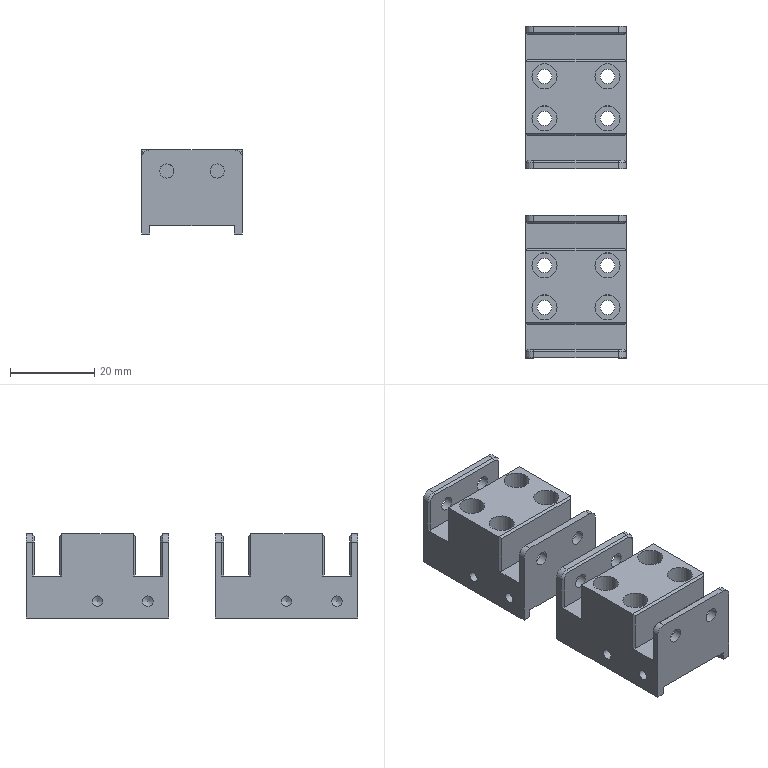CAM job | NX | 3-axis milling, drilling | part box 24 x 79 x 20 mm | stock box 25 x 84 x 25 mm
Tools:
number,name,description,diameter,corner_radius,flute_length,length,flutes
4,D4,平底铣刀-粗,4.0,0.0,25.0,75.0,2
9,D10,平底铣刀-粗,10.0,0.0,35.0,75.0,2
11,D4-J,平底铣刀-精,4.0,0.0,50.0,75.0,2
10,D10-J,平底铣刀-精,10.0,0.0,35.0,75.0,2
18,D4R0.5,圆鼻刀-粗,4.0,0.5,50.0,75.0,2
1,D80R0.8飞刀,圆鼻刀-粗,80.0,0.8,50.0,75.0,2
1,D80R0.8飞刀-J,圆鼻刀-精,80.0,0.8,50.0,75.0,2
2,D6倒角刀,倒角刀,6.0,0.0,3.0,25.0,2
13,ZT3.4,钻头,3.4,0.0,35.0,50.0,2
Operations:
program,operation,operation_type,tool,method,geometry_group,spindle_rpm,surface_speed,feed_per_tooth,feed_cut,feed_plunge,cut_length_mm,path_length_mm,cut_time_min,machine_time_min
B,FLOORWALL_FACEMILL1ROUGH_COPY,VolumeBased25DMillingOperation,D80R0.8飞刀,LAYERROUGH-DEPTHK-STEPG,W-B,2800.0,703.696,0.5357,3000.0,100.0,1684.746,3348.967,0.5616,0.728
B,FLOORWALL_FACEMILL1FINISH_COPY,VolumeBased25DMillingOperation,D80R0.8飞刀-J,SIDEFINISH-DEPTHK-STEPG,W-B,4000.0,1005.28,0.125,1000.0,100.0,186.998,222.998,0.187,0.1906
B,FLOORWALL_LAYERROUGH-MID_COPY,VolumeBased25DMillingOperation,D10,LAYERROUGH-DEPTHK-STEPG,W-B,8000.0,251.327,0.1875,3000.0,100.0,1507.802,1545.965,0.5026,0.5064
B,FLOORWALL_FLOORFINISH-MID_COPY,VolumeBased25DMillingOperation,D10-J,FINISHSTEPDEPTHOFF,W-B,8000.0,251.32,0.0625,1000.0,100.0,197.366,227.366,0.1974,0.2004
B,PLANEDEBURR6X45L_COPY,SurfaceContour,D6倒角刀,CLIMB_CHAMFER-DEPTH0-STEPG,W-B,6500.0,122.519,0.1154,1500.0,100.0,396.385,831.625,0.2643,0.3078
B,FLOORWALL_SIDEFINISH-MID-SELFLOOR_COPY,VolumeBased25DMillingOperation,D10-J,SIDEFINISH-DEPTHK-STEPG,W-B,8000.0,251.32,0.0625,1000.0,100.0,198.29,229.29,0.1983,0.2014
A,TOPROUGH,FaceMilling,D80R0.8飞刀,LAYERROUGH-DEPTHK-STEPG,W-A,4000.0,1005.31,0.375,3000.0,100.0,173.0,208.8,0.0577,0.0612
A,TOP,FaceMilling,D80R0.8飞刀,SIDEFINISH-DEPTHK-STEPG,W-A,4000.0,1005.31,0.125,1000.0,100.0,173.0,209.0,0.173,0.1766
A,PROFILEROUGH_2,VolumeBased25DMillingOperation,D10,METHOD,W-A,8000.0,251.327,0.3125,5000.0,80.0,12734.875,12897.975,2.547,2.563
A,CSINKSPOT-DEPTH0.8,Operation,D6倒角刀,NONE,W-A,8000.0,150.796,0.0312,500.0,90.0,14.4,181.08,0.0288,0.0455
A,CSINK-DRILL0SEG,Operation,ZT3.4,NONE,W-A,2800.0,29.908,0.0179,100.0,90.0,176.172,504.624,1.762,1.795
A,FLOORWALLROUGH_1,VolumeBased25DMillingOperation,D4,METHOD,W-A,6000.0,75.398,0.1,1200.0,100.0,4757.645,5320.5,3.965,4.021
A,FLOORWALLROUGH_2,VolumeBased25DMillingOperation,D4,METHOD,W-A,6000.0,75.398,0.1,1200.0,100.0,4757.645,5319.506,3.965,4.021
A,HOLEROUGHD4_1,CylinderMilling,D4,NONE,W-A,8000.0,100.531,0.075,1200.0,100.0,2106.473,2634.501,1.755,1.808
A,HOLEFINISHD4_1,CylinderMilling,D4-J,FINISHSTEPDEPTHOFF,W-A,8000.0,100.531,0.0312,500.0,100.0,248.006,776.033,0.496,0.5488
A,FLOORSIDEFINISH_3,VolumeBased25DMillingOperation,D4-J,METHOD,W-A,6000.0,113.0,0.2083,1200.0,100.0,261.8,767.141,0.2182,0.2687
A,FLOORSIDEFINISH_4,VolumeBased25DMillingOperation,D4-J,METHOD,W-A,6000.0,113.0,0.2083,1200.0,100.0,261.8,767.201,0.2182,0.2687
A,CONTOURFINISHRECIPCLIMB_COPY,ZLevelMilling,D4R0.5,CONTOURCLIMB-DEPTHK-STEPG,W-A,7000.0,131.947,0.2857,4000.0,100.0,2549.079,2923.801,0.6373,0.6747
A,SELBODYONLY,SurfaceContour,D6倒角刀,METHOD,W-A,8000.0,150.796,0.1875,3000.0,100.0,231.558,559.712,0.0772,0.11
A,FLOORWALLCHAMFER_COPY,VolumeBased25DMillingOperation,D6倒角刀,CLIMB_CHAMFER-DEPTH0-STEPG,W-A,6500.0,122.519,0.1154,1500.0,100.0,165.014,396.027,0.11,0.1331
A,MILLCHAMFER_1,PlanarMilling,D6倒角刀,NONE,W-A,8000.0,150.796,0.0312,500.0,100.0,221.477,618.589,0.443,0.4827
A,FLOORWALLCHAMFER_COPY_1,VolumeBased25DMillingOperation,D6倒角刀,CLIMB_CHAMFER-DEPTH0-STEPG,W-A,6500.0,122.519,0.1154,1500.0,100.0,144.739,369.139,0.0965,0.1189
A,PROFILESEMIFINISH_2,VolumeBased25DMillingOperation,D10-J,METHOD,W-A,8000.0,251.327,0.0625,1000.0,100.0,617.734,894.948,0.6177,0.6455